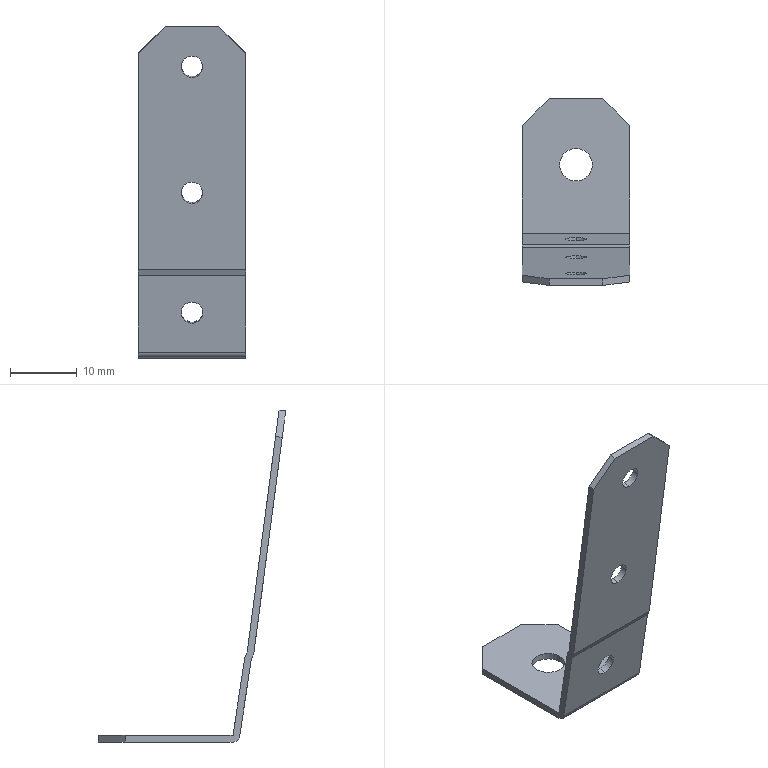Part | SolidWorks | features BaseBody 1 | 1 solid | 25 faces | box 16 x 28.013 x 49.636 mm | volume 1045 mm3 | plane 16 | cylinder 9 | commonest cylinder face diameters 3.2 x6 4.9 x2 2 x1
STEP:
#1=CARTESIAN_POINT('',(-142.,-118.576,-942.719));
#2=VERTEX_POINT('',#1);
#3=CARTESIAN_POINT('',(-142.,-118.159,-945.892));
#4=VERTEX_POINT('',#3);
#5=CARTESIAN_POINT('',(-142.,-118.576,-942.719));
#6=CARTESIAN_POINT('',(-145.2,-118.576,-942.719));
#7=CARTESIAN_POINT('',(-145.2,-118.159,-945.892));
#8=CARTESIAN_POINT('',(-142.,-118.159,-945.892));
#9=(BOUNDED_CURVE()B_SPLINE_CURVE(3,(#5,#6,#7,#8),.UNSPECIFIED.,.F.,.F.)B_SPLINE_CURVE_WITH_KNOTS((4,4),(0.,3.142),.UNSPECIFIED.)CURVE()GEOMETRIC_REPRESENTATION_ITEM()RATIONAL_B_SPLINE_CURVE((1.,0.3333,0.3333,1.))REPRESENTATION_ITEM(''));
#10=EDGE_CURVE('',#2,#4,#9,.T.);
#11=ORIENTED_EDGE('',*,*,#10,.T.);
#12=CARTESIAN_POINT('',(-142.,-117.17,-945.743));
#13=VERTEX_POINT('',#12);
#14=CARTESIAN_POINT('',(-142.,-118.165,-945.893));
#15=DIRECTION('',(0.,0.9888,0.1494));
#16=VECTOR('',#15,1000.);
#17=LINE('',#14,#16);
#18=EDGE_CURVE('',#4,#13,#17,.T.);
#19=ORIENTED_EDGE('',*,*,#18,.T.);
#20=CARTESIAN_POINT('',(-142.,-117.587,-942.57));
#21=VERTEX_POINT('',#20);
#22=CARTESIAN_POINT('',(-142.,-117.17,-945.743));
#23=CARTESIAN_POINT('',(-145.2,-117.17,-945.743));
#24=CARTESIAN_POINT('',(-145.2,-117.587,-942.57));
#25=CARTESIAN_POINT('',(-142.,-117.587,-942.57));
#26=(BOUNDED_CURVE()B_SPLINE_CURVE(3,(#22,#23,#24,#25),.UNSPECIFIED.,.F.,.F.)B_SPLINE_CURVE_WITH_KNOTS((4,4),(3.142,6.283),.UNSPECIFIED.)CURVE()GEOMETRIC_REPRESENTATION_ITEM()RATIONAL_B_SPLINE_CURVE((1.,0.3333,0.3333,1.))REPRESENTATION_ITEM(''));
#27=EDGE_CURVE('',#13,#21,#26,.T.);
#28=ORIENTED_EDGE('',*,*,#27,.T.);
#29=CARTESIAN_POINT('',(-142.,-118.643,-942.729));
#30=DIRECTION('',(0.,0.9888,0.1494));
#31=VECTOR('',#30,1000.);
#32=LINE('',#29,#31);
#33=EDGE_CURVE('',#2,#21,#32,.T.);
#34=ORIENTED_EDGE('',*,*,#33,.F.);
#35=EDGE_LOOP('',(#11,#19,#28,#34));
#36=FACE_OUTER_BOUND('',#35,.T.);
#37=CARTESIAN_POINT('',(-142.,-118.404,-944.311));
#38=DIRECTION('',(0.,0.9888,0.1494));
#39=DIRECTION('',(0.,-0.1494,0.9888));
#40=AXIS2_PLACEMENT_3D('',#37,#38,#39);
#41=CYLINDRICAL_SURFACE('',#40,1.6);
#42=ADVANCED_FACE('',(#36),#41,.F.);
#43=CARTESIAN_POINT('',(-142.,-121.052,-923.878));
#44=VERTEX_POINT('',#43);
#45=CARTESIAN_POINT('',(-142.,-120.635,-927.051));
#46=VERTEX_POINT('',#45);
#47=CARTESIAN_POINT('',(-142.,-121.052,-923.878));
#48=CARTESIAN_POINT('',(-145.2,-121.052,-923.878));
#49=CARTESIAN_POINT('',(-145.2,-120.635,-927.051));
#50=CARTESIAN_POINT('',(-142.,-120.635,-927.051));
#51=(BOUNDED_CURVE()B_SPLINE_CURVE(3,(#47,#48,#49,#50),.UNSPECIFIED.,.F.,.T.)B_SPLINE_CURVE_WITH_KNOTS((4,4),(0.,3.142),.UNSPECIFIED.)CURVE()GEOMETRIC_REPRESENTATION_ITEM()RATIONAL_B_SPLINE_CURVE((1.,0.3333,0.3333,1.))REPRESENTATION_ITEM(''));
#52=EDGE_CURVE('',#44,#46,#51,.T.);
#53=ORIENTED_EDGE('',*,*,#52,.T.);
#54=CARTESIAN_POINT('',(-142.,-119.646,-926.902));
#55=VERTEX_POINT('',#54);
#56=CARTESIAN_POINT('',(-142.,-120.641,-927.052));
#57=DIRECTION('',(0.,0.9888,0.1494));
#58=VECTOR('',#57,1000.);
#59=LINE('',#56,#58);
#60=EDGE_CURVE('',#46,#55,#59,.T.);
#61=ORIENTED_EDGE('',*,*,#60,.T.);
#62=CARTESIAN_POINT('',(-142.,-120.063,-923.728));
#63=VERTEX_POINT('',#62);
#64=CARTESIAN_POINT('',(-142.,-119.646,-926.902));
#65=CARTESIAN_POINT('',(-145.2,-119.646,-926.902));
#66=CARTESIAN_POINT('',(-145.2,-120.063,-923.728));
#67=CARTESIAN_POINT('',(-142.,-120.063,-923.728));
#68=(BOUNDED_CURVE()B_SPLINE_CURVE(3,(#64,#65,#66,#67),.UNSPECIFIED.,.F.,.F.)B_SPLINE_CURVE_WITH_KNOTS((4,4),(3.142,6.283),.UNSPECIFIED.)CURVE()GEOMETRIC_REPRESENTATION_ITEM()RATIONAL_B_SPLINE_CURVE((1.,0.3333,0.3333,1.))REPRESENTATION_ITEM(''));
#69=EDGE_CURVE('',#55,#63,#68,.T.);
#70=ORIENTED_EDGE('',*,*,#69,.T.);
#71=CARTESIAN_POINT('',(-142.,-121.119,-923.888));
#72=DIRECTION('',(0.,0.9888,0.1494));
#73=VECTOR('',#72,1000.);
#74=LINE('',#71,#73);
#75=EDGE_CURVE('',#44,#63,#74,.T.);
#76=ORIENTED_EDGE('',*,*,#75,.F.);
#77=EDGE_LOOP('',(#53,#61,#70,#76));
#78=FACE_OUTER_BOUND('',#77,.T.);
#79=CARTESIAN_POINT('',(-142.,-120.88,-925.47));
#80=DIRECTION('',(0.,0.9888,0.1494));
#81=DIRECTION('',(0.,-0.1494,0.9888));
#82=AXIS2_PLACEMENT_3D('',#79,#80,#81);
#83=CYLINDRICAL_SURFACE('',#82,1.6);
#84=ADVANCED_FACE('',(#78),#83,.F.);
#85=CARTESIAN_POINT('',(-142.,-115.879,-960.636));
#86=VERTEX_POINT('',#85);
#87=CARTESIAN_POINT('',(-142.,-115.401,-963.8));
#88=VERTEX_POINT('',#87);
#89=CARTESIAN_POINT('',(-142.,-115.64,-962.218));
#90=DIRECTION('',(0.,-0.9888,-0.1494));
#91=DIRECTION('',(0.,-0.1494,0.9888));
#92=AXIS2_PLACEMENT_3D('',#89,#90,#91);
#93=CIRCLE('',#92,1.6);
#94=EDGE_CURVE('',#86,#88,#93,.T.);
#95=ORIENTED_EDGE('',*,*,#94,.T.);
#96=CARTESIAN_POINT('',(-142.,-114.412,-963.65));
#97=VERTEX_POINT('',#96);
#98=CARTESIAN_POINT('',(-142.,-115.401,-963.8));
#99=DIRECTION('',(0.,0.9888,0.1494));
#100=VECTOR('',#99,1000.);
#101=LINE('',#98,#100);
#102=EDGE_CURVE('',#88,#97,#101,.T.);
#103=ORIENTED_EDGE('',*,*,#102,.T.);
#104=CARTESIAN_POINT('',(-142.,-114.89,-960.486));
#105=VERTEX_POINT('',#104);
#106=CARTESIAN_POINT('',(-142.,-114.651,-962.068));
#107=DIRECTION('',(0.,0.9888,0.1494));
#108=DIRECTION('',(0.,-0.1494,0.9888));
#109=AXIS2_PLACEMENT_3D('',#106,#107,#108);
#110=CIRCLE('',#109,1.6);
#111=EDGE_CURVE('',#97,#105,#110,.T.);
#112=ORIENTED_EDGE('',*,*,#111,.T.);
#113=CARTESIAN_POINT('',(-142.,-115.879,-960.636));
#114=DIRECTION('',(0.,0.9888,0.1494));
#115=VECTOR('',#114,1000.);
#116=LINE('',#113,#115);
#117=EDGE_CURVE('',#86,#105,#116,.T.);
#118=ORIENTED_EDGE('',*,*,#117,.F.);
#119=EDGE_LOOP('',(#95,#103,#112,#118));
#120=FACE_OUTER_BOUND('',#119,.T.);
#121=CARTESIAN_POINT('',(-142.,-115.64,-962.218));
#122=DIRECTION('',(0.,0.9888,0.1494));
#123=DIRECTION('',(0.,-0.1494,0.9888));
#124=AXIS2_PLACEMENT_3D('',#121,#122,#123);
#125=CYLINDRICAL_SURFACE('',#124,1.6);
#126=ADVANCED_FACE('',(#120),#125,.F.);
#127=CARTESIAN_POINT('',(-139.55,-103.5,-969.001));
#128=VERTEX_POINT('',#127);
#129=CARTESIAN_POINT('',(-144.45,-103.5,-969.001));
#130=VERTEX_POINT('',#129);
#131=CARTESIAN_POINT('',(-142.,-103.5,-969.001));
#132=DIRECTION('',(0.,0.,-1.));
#133=DIRECTION('',(1.,0.,0.));
#134=AXIS2_PLACEMENT_3D('',#131,#132,#133);
#135=CIRCLE('',#134,2.45);
#136=EDGE_CURVE('',#128,#130,#135,.T.);
#137=ORIENTED_EDGE('',*,*,#136,.T.);
#138=CARTESIAN_POINT('',(-144.45,-103.5,-968.001));
#139=VERTEX_POINT('',#138);
#140=CARTESIAN_POINT('',(-144.45,-103.5,-969.001));
#141=DIRECTION('',(0.,0.,1.));
#142=VECTOR('',#141,1000.);
#143=LINE('',#140,#142);
#144=EDGE_CURVE('',#130,#139,#143,.T.);
#145=ORIENTED_EDGE('',*,*,#144,.T.);
#146=CARTESIAN_POINT('',(-139.55,-103.5,-968.001));
#147=VERTEX_POINT('',#146);
#148=CARTESIAN_POINT('',(-142.,-103.5,-968.001));
#149=DIRECTION('',(0.,0.,1.));
#150=DIRECTION('',(1.,0.,0.));
#151=AXIS2_PLACEMENT_3D('',#148,#149,#150);
#152=CIRCLE('',#151,2.45);
#153=EDGE_CURVE('',#139,#147,#152,.T.);
#154=ORIENTED_EDGE('',*,*,#153,.T.);
#155=CARTESIAN_POINT('',(-139.55,-103.5,-969.001));
#156=DIRECTION('',(0.,0.,1.));
#157=VECTOR('',#156,1000.);
#158=LINE('',#155,#157);
#159=EDGE_CURVE('',#128,#147,#158,.T.);
#160=ORIENTED_EDGE('',*,*,#159,.F.);
#161=EDGE_LOOP('',(#137,#145,#154,#160));
#162=FACE_OUTER_BOUND('',#161,.T.);
#163=CARTESIAN_POINT('',(-142.,-103.5,-969.001));
#164=DIRECTION('',(0.,0.,1.));
#165=DIRECTION('',(1.,0.,0.));
#166=AXIS2_PLACEMENT_3D('',#163,#164,#165);
#167=CYLINDRICAL_SURFACE('',#166,2.45);
#168=ADVANCED_FACE('',(#162),#167,.F.);
#169=ORIENTED_EDGE('',*,*,#18,.F.);
#170=CARTESIAN_POINT('',(-142.,-118.159,-945.892));
#171=CARTESIAN_POINT('',(-138.8,-118.159,-945.892));
#172=CARTESIAN_POINT('',(-138.8,-118.576,-942.719));
#173=CARTESIAN_POINT('',(-142.,-118.576,-942.719));
#174=(BOUNDED_CURVE()B_SPLINE_CURVE(3,(#170,#171,#172,#173),.UNSPECIFIED.,.F.,.F.)B_SPLINE_CURVE_WITH_KNOTS((4,4),(3.142,6.283),.UNSPECIFIED.)CURVE()GEOMETRIC_REPRESENTATION_ITEM()RATIONAL_B_SPLINE_CURVE((1.,0.3333,0.3333,1.))REPRESENTATION_ITEM(''));
#175=EDGE_CURVE('',#4,#2,#174,.T.);
#176=ORIENTED_EDGE('',*,*,#175,.T.);
#177=ORIENTED_EDGE('',*,*,#33,.T.);
#178=CARTESIAN_POINT('',(-142.,-117.587,-942.57));
#179=CARTESIAN_POINT('',(-138.8,-117.587,-942.57));
#180=CARTESIAN_POINT('',(-138.8,-117.17,-945.743));
#181=CARTESIAN_POINT('',(-142.,-117.17,-945.743));
#182=(BOUNDED_CURVE()B_SPLINE_CURVE(3,(#178,#179,#180,#181),.UNSPECIFIED.,.F.,.F.)B_SPLINE_CURVE_WITH_KNOTS((4,4),(0.,3.142),.UNSPECIFIED.)CURVE()GEOMETRIC_REPRESENTATION_ITEM()RATIONAL_B_SPLINE_CURVE((1.,0.3333,0.3333,1.))REPRESENTATION_ITEM(''));
#183=EDGE_CURVE('',#21,#13,#182,.T.);
#184=ORIENTED_EDGE('',*,*,#183,.T.);
#185=EDGE_LOOP('',(#169,#176,#177,#184));
#186=FACE_OUTER_BOUND('',#185,.T.);
#187=CARTESIAN_POINT('',(-142.,-118.404,-944.311));
#188=DIRECTION('',(0.,0.9888,0.1494));
#189=DIRECTION('',(0.,-0.1494,0.9888));
#190=AXIS2_PLACEMENT_3D('',#187,#188,#189);
#191=CYLINDRICAL_SURFACE('',#190,1.6);
#192=ADVANCED_FACE('',(#186),#191,.F.);
#193=CARTESIAN_POINT('',(-142.,-120.063,-923.728));
#194=CARTESIAN_POINT('',(-138.8,-120.063,-923.728));
#195=CARTESIAN_POINT('',(-138.8,-119.646,-926.902));
#196=CARTESIAN_POINT('',(-142.,-119.646,-926.902));
#197=(BOUNDED_CURVE()B_SPLINE_CURVE(3,(#193,#194,#195,#196),.UNSPECIFIED.,.F.,.T.)B_SPLINE_CURVE_WITH_KNOTS((4,4),(0.,3.142),.UNSPECIFIED.)CURVE()GEOMETRIC_REPRESENTATION_ITEM()RATIONAL_B_SPLINE_CURVE((1.,0.3333,0.3333,1.))REPRESENTATION_ITEM(''));
#198=EDGE_CURVE('',#63,#55,#197,.T.);
#199=ORIENTED_EDGE('',*,*,#198,.F.);
#200=ORIENTED_EDGE('',*,*,#69,.F.);
#201=EDGE_LOOP('',(#199,#200));
#202=FACE_BOUND('',#201,.T.);
#203=ORIENTED_EDGE('',*,*,#183,.F.);
#204=ORIENTED_EDGE('',*,*,#27,.F.);
#205=EDGE_LOOP('',(#203,#204));
#206=FACE_BOUND('',#205,.T.);
#207=CARTESIAN_POINT('',(-134.,-120.116,-923.331));
#208=VERTEX_POINT('',#207);
#209=CARTESIAN_POINT('',(-138.,-120.637,-919.365));
#210=VERTEX_POINT('',#209);
#211=CARTESIAN_POINT('',(-138.,-120.637,-919.365));
#212=DIRECTION('',(-0.7071,-0.09215,0.7011));
#213=VECTOR('',#212,1000.);
#214=LINE('',#211,#213);
#215=EDGE_CURVE('',#208,#210,#214,.T.);
#216=ORIENTED_EDGE('',*,*,#215,.F.);
#217=CARTESIAN_POINT('',(-134.,-115.881,-955.544));
#218=VERTEX_POINT('',#217);
#219=CARTESIAN_POINT('',(-134.,-118.259,-937.455));
#220=DIRECTION('',(0.,-0.1303,0.9915));
#221=VECTOR('',#220,1000.);
#222=LINE('',#219,#221);
#223=EDGE_CURVE('',#218,#208,#222,.T.);
#224=ORIENTED_EDGE('',*,*,#223,.F.);
#225=CARTESIAN_POINT('',(-150.,-115.881,-955.544));
#226=VERTEX_POINT('',#225);
#227=CARTESIAN_POINT('',(-142.,-115.881,-955.544));
#228=DIRECTION('',(1.,0.,0.));
#229=VECTOR('',#228,1000.);
#230=LINE('',#227,#229);
#231=EDGE_CURVE('',#226,#218,#230,.T.);
#232=ORIENTED_EDGE('',*,*,#231,.F.);
#233=CARTESIAN_POINT('',(-150.,-120.116,-923.331));
#234=VERTEX_POINT('',#233);
#235=CARTESIAN_POINT('',(-150.,-118.259,-937.455));
#236=DIRECTION('',(0.,0.1303,-0.9915));
#237=VECTOR('',#236,1000.);
#238=LINE('',#235,#237);
#239=EDGE_CURVE('',#234,#226,#238,.T.);
#240=ORIENTED_EDGE('',*,*,#239,.F.);
#241=CARTESIAN_POINT('',(-146.,-120.637,-919.365));
#242=VERTEX_POINT('',#241);
#243=CARTESIAN_POINT('',(-150.,-120.116,-923.331));
#244=DIRECTION('',(-0.7071,0.09215,-0.7011));
#245=VECTOR('',#244,1000.);
#246=LINE('',#243,#245);
#247=EDGE_CURVE('',#242,#234,#246,.T.);
#248=ORIENTED_EDGE('',*,*,#247,.F.);
#249=CARTESIAN_POINT('',(-142.,-120.637,-919.365));
#250=DIRECTION('',(-1.,0.,0.));
#251=VECTOR('',#250,1000.);
#252=LINE('',#249,#251);
#253=EDGE_CURVE('',#210,#242,#252,.T.);
#254=ORIENTED_EDGE('',*,*,#253,.F.);
#255=EDGE_LOOP('',(#216,#224,#232,#240,#248,#254));
#256=FACE_OUTER_BOUND('',#255,.T.);
#257=CARTESIAN_POINT('',(-150.,-120.637,-919.365));
#258=DIRECTION('',(0.,-0.9915,-0.1303));
#259=DIRECTION('',(0.,0.1303,-0.9915));
#260=AXIS2_PLACEMENT_3D('',#257,#258,#259);
#261=PLANE('',#260);
#262=ADVANCED_FACE('',(#202,#206,#256),#261,.F.);
#263=ORIENTED_EDGE('',*,*,#52,.F.);
#264=CARTESIAN_POINT('',(-142.,-120.635,-927.051));
#265=CARTESIAN_POINT('',(-138.8,-120.635,-927.051));
#266=CARTESIAN_POINT('',(-138.8,-121.052,-923.878));
#267=CARTESIAN_POINT('',(-142.,-121.052,-923.878));
#268=(BOUNDED_CURVE()B_SPLINE_CURVE(3,(#264,#265,#266,#267),.UNSPECIFIED.,.F.,.F.)B_SPLINE_CURVE_WITH_KNOTS((4,4),(3.142,6.283),.UNSPECIFIED.)CURVE()GEOMETRIC_REPRESENTATION_ITEM()RATIONAL_B_SPLINE_CURVE((1.,0.3333,0.3333,1.))REPRESENTATION_ITEM(''));
#269=EDGE_CURVE('',#46,#44,#268,.T.);
#270=ORIENTED_EDGE('',*,*,#269,.F.);
#271=EDGE_LOOP('',(#263,#270));
#272=FACE_BOUND('',#271,.T.);
#273=ORIENTED_EDGE('',*,*,#10,.F.);
#274=ORIENTED_EDGE('',*,*,#175,.F.);
#275=EDGE_LOOP('',(#273,#274));
#276=FACE_BOUND('',#275,.T.);
#277=CARTESIAN_POINT('',(-138.,-121.628,-919.495));
#278=VERTEX_POINT('',#277);
#279=CARTESIAN_POINT('',(-134.,-121.107,-923.461));
#280=VERTEX_POINT('',#279);
#281=CARTESIAN_POINT('',(-138.,-121.628,-919.495));
#282=DIRECTION('',(0.7071,0.09215,-0.7011));
#283=VECTOR('',#282,1000.);
#284=LINE('',#281,#283);
#285=EDGE_CURVE('',#278,#280,#284,.T.);
#286=ORIENTED_EDGE('',*,*,#285,.F.);
#287=CARTESIAN_POINT('',(-146.,-121.628,-919.495));
#288=VERTEX_POINT('',#287);
#289=CARTESIAN_POINT('',(-142.,-121.628,-919.495));
#290=DIRECTION('',(1.,0.,0.));
#291=VECTOR('',#290,1000.);
#292=LINE('',#289,#291);
#293=EDGE_CURVE('',#288,#278,#292,.T.);
#294=ORIENTED_EDGE('',*,*,#293,.F.);
#295=CARTESIAN_POINT('',(-150.,-121.107,-923.461));
#296=VERTEX_POINT('',#295);
#297=CARTESIAN_POINT('',(-150.,-121.107,-923.461));
#298=DIRECTION('',(0.7071,-0.09215,0.7011));
#299=VECTOR('',#298,1000.);
#300=LINE('',#297,#299);
#301=EDGE_CURVE('',#296,#288,#300,.T.);
#302=ORIENTED_EDGE('',*,*,#301,.F.);
#303=CARTESIAN_POINT('',(-150.,-116.854,-955.821));
#304=VERTEX_POINT('',#303);
#305=CARTESIAN_POINT('',(-150.,-119.241,-937.658));
#306=DIRECTION('',(0.,-0.1303,0.9915));
#307=VECTOR('',#306,1000.);
#308=LINE('',#305,#307);
#309=EDGE_CURVE('',#304,#296,#308,.T.);
#310=ORIENTED_EDGE('',*,*,#309,.F.);
#311=CARTESIAN_POINT('',(-134.,-116.854,-955.821));
#312=VERTEX_POINT('',#311);
#313=CARTESIAN_POINT('',(-142.,-116.854,-955.821));
#314=DIRECTION('',(-1.,0.,0.));
#315=VECTOR('',#314,1000.);
#316=LINE('',#313,#315);
#317=EDGE_CURVE('',#312,#304,#316,.T.);
#318=ORIENTED_EDGE('',*,*,#317,.F.);
#319=CARTESIAN_POINT('',(-134.,-119.241,-937.658));
#320=DIRECTION('',(0.,0.1303,-0.9915));
#321=VECTOR('',#320,1000.);
#322=LINE('',#319,#321);
#323=EDGE_CURVE('',#280,#312,#322,.T.);
#324=ORIENTED_EDGE('',*,*,#323,.F.);
#325=EDGE_LOOP('',(#286,#294,#302,#310,#318,#324));
#326=FACE_OUTER_BOUND('',#325,.T.);
#327=CARTESIAN_POINT('',(-150.,-116.854,-955.821));
#328=DIRECTION('',(0.,0.9915,0.1303));
#329=DIRECTION('',(0.,-0.1303,0.9915));
#330=AXIS2_PLACEMENT_3D('',#327,#328,#329);
#331=PLANE('',#330);
#332=ADVANCED_FACE('',(#272,#276,#326),#331,.F.);
#333=ORIENTED_EDGE('',*,*,#60,.F.);
#334=ORIENTED_EDGE('',*,*,#269,.T.);
#335=ORIENTED_EDGE('',*,*,#75,.T.);
#336=ORIENTED_EDGE('',*,*,#198,.T.);
#337=EDGE_LOOP('',(#333,#334,#335,#336));
#338=FACE_OUTER_BOUND('',#337,.T.);
#339=CARTESIAN_POINT('',(-142.,-120.88,-925.47));
#340=DIRECTION('',(0.,0.9888,0.1494));
#341=DIRECTION('',(0.,-0.1494,0.9888));
#342=AXIS2_PLACEMENT_3D('',#339,#340,#341);
#343=CYLINDRICAL_SURFACE('',#342,1.6);
#344=ADVANCED_FACE('',(#338),#343,.F.);
#345=CARTESIAN_POINT('',(-138.,-121.133,-919.43));
#346=DIRECTION('',(0.,-0.9915,-0.1303));
#347=VECTOR('',#346,1000.);
#348=LINE('',#345,#347);
#349=EDGE_CURVE('',#210,#278,#348,.T.);
#350=ORIENTED_EDGE('',*,*,#349,.F.);
#351=ORIENTED_EDGE('',*,*,#253,.T.);
#352=CARTESIAN_POINT('',(-146.,-121.133,-919.43));
#353=DIRECTION('',(0.,0.9915,0.1303));
#354=VECTOR('',#353,1000.);
#355=LINE('',#352,#354);
#356=EDGE_CURVE('',#288,#242,#355,.T.);
#357=ORIENTED_EDGE('',*,*,#356,.F.);
#358=ORIENTED_EDGE('',*,*,#293,.T.);
#359=EDGE_LOOP('',(#350,#351,#357,#358));
#360=FACE_OUTER_BOUND('',#359,.T.);
#361=CARTESIAN_POINT('',(-146.,-121.628,-919.495));
#362=DIRECTION('',(0.,0.1303,-0.9915));
#363=DIRECTION('',(0.,0.9915,0.1303));
#364=AXIS2_PLACEMENT_3D('',#361,#362,#363);
#365=PLANE('',#364);
#366=ADVANCED_FACE('',(#360),#365,.F.);
#367=ORIENTED_EDGE('',*,*,#215,.T.);
#368=ORIENTED_EDGE('',*,*,#349,.T.);
#369=ORIENTED_EDGE('',*,*,#285,.T.);
#370=CARTESIAN_POINT('',(-134.,-120.611,-923.396));
#371=DIRECTION('',(0.,0.9915,0.1303));
#372=VECTOR('',#371,1000.);
#373=LINE('',#370,#372);
#374=EDGE_CURVE('',#280,#208,#373,.T.);
#375=ORIENTED_EDGE('',*,*,#374,.T.);
#376=EDGE_LOOP('',(#367,#368,#369,#375));
#377=FACE_OUTER_BOUND('',#376,.T.);
#378=CARTESIAN_POINT('',(-138.,-120.637,-919.365));
#379=DIRECTION('',(0.7071,-0.09215,0.7011));
#380=DIRECTION('',(0.,-0.9915,-0.1303));
#381=AXIS2_PLACEMENT_3D('',#378,#379,#380);
#382=PLANE('',#381);
#383=ADVANCED_FACE('',(#377),#382,.T.);
#384=CARTESIAN_POINT('',(-134.,-113.755,-968.001));
#385=VERTEX_POINT('',#384);
#386=CARTESIAN_POINT('',(-134.,-115.513,-956.362));
#387=VERTEX_POINT('',#386);
#388=CARTESIAN_POINT('',(-134.,-113.755,-968.001));
#389=DIRECTION('',(0.,-0.1494,0.9888));
#390=VECTOR('',#389,1000.);
#391=LINE('',#388,#390);
#392=EDGE_CURVE('',#385,#387,#391,.T.);
#393=ORIENTED_EDGE('',*,*,#392,.T.);
#394=CARTESIAN_POINT('',(-134.,-115.513,-956.362));
#395=DIRECTION('',(0.,-0.4107,0.9118));
#396=VECTOR('',#395,1000.);
#397=LINE('',#394,#396);
#398=EDGE_CURVE('',#387,#218,#397,.T.);
#399=ORIENTED_EDGE('',*,*,#398,.T.);
#400=ORIENTED_EDGE('',*,*,#223,.T.);
#401=ORIENTED_EDGE('',*,*,#374,.F.);
#402=ORIENTED_EDGE('',*,*,#323,.T.);
#403=CARTESIAN_POINT('',(-134.,-116.481,-956.647));
#404=VERTEX_POINT('',#403);
#405=CARTESIAN_POINT('',(-134.,-116.854,-955.821));
#406=DIRECTION('',(0.,0.4107,-0.9118));
#407=VECTOR('',#406,1000.);
#408=LINE('',#405,#407);
#409=EDGE_CURVE('',#312,#404,#408,.T.);
#410=ORIENTED_EDGE('',*,*,#409,.T.);
#411=CARTESIAN_POINT('',(-134.,-114.744,-968.15));
#412=VERTEX_POINT('',#411);
#413=CARTESIAN_POINT('',(-134.,-116.481,-956.647));
#414=DIRECTION('',(0.,0.1494,-0.9888));
#415=VECTOR('',#414,1000.);
#416=LINE('',#413,#415);
#417=EDGE_CURVE('',#404,#412,#416,.T.);
#418=ORIENTED_EDGE('',*,*,#417,.T.);
#419=CARTESIAN_POINT('',(-134.,-113.755,-969.001));
#420=VERTEX_POINT('',#419);
#421=CARTESIAN_POINT('',(-134.,-113.755,-968.001));
#422=DIRECTION('',(1.,0.,0.));
#423=DIRECTION('',(0.,0.,-1.));
#424=AXIS2_PLACEMENT_3D('',#421,#422,#423);
#425=CIRCLE('',#424,1.);
#426=EDGE_CURVE('',#412,#420,#425,.T.);
#427=ORIENTED_EDGE('',*,*,#426,.T.);
#428=CARTESIAN_POINT('',(-134.,-97.615,-969.001));
#429=VERTEX_POINT('',#428);
#430=CARTESIAN_POINT('',(-134.,-109.432,-969.001));
#431=DIRECTION('',(0.,1.,0.));
#432=VECTOR('',#431,1000.);
#433=LINE('',#430,#432);
#434=EDGE_CURVE('',#420,#429,#433,.T.);
#435=ORIENTED_EDGE('',*,*,#434,.T.);
#436=CARTESIAN_POINT('',(-134.,-97.615,-968.001));
#437=VERTEX_POINT('',#436);
#438=CARTESIAN_POINT('',(-134.,-97.615,-968.501));
#439=DIRECTION('',(0.,0.,-1.));
#440=VECTOR('',#439,1000.);
#441=LINE('',#438,#440);
#442=EDGE_CURVE('',#437,#429,#441,.T.);
#443=ORIENTED_EDGE('',*,*,#442,.F.);
#444=CARTESIAN_POINT('',(-134.,-109.432,-968.001));
#445=DIRECTION('',(0.,-1.,0.));
#446=VECTOR('',#445,1000.);
#447=LINE('',#444,#446);
#448=EDGE_CURVE('',#437,#385,#447,.T.);
#449=ORIENTED_EDGE('',*,*,#448,.T.);
#450=EDGE_LOOP('',(#393,#399,#400,#401,#402,#410,#418,#427,#435,#443,#449));
#451=FACE_OUTER_BOUND('',#450,.T.);
#452=CARTESIAN_POINT('',(-134.,-121.248,-923.057));
#453=DIRECTION('',(1.,0.,0.));
#454=DIRECTION('',(0.,0.,-1.));
#455=AXIS2_PLACEMENT_3D('',#452,#453,#454);
#456=PLANE('',#455);
#457=ADVANCED_FACE('',(#451),#456,.T.);
#458=CARTESIAN_POINT('',(-150.,-115.513,-956.362));
#459=VERTEX_POINT('',#458);
#460=CARTESIAN_POINT('',(-142.,-115.513,-956.362));
#461=DIRECTION('',(1.,0.,0.));
#462=VECTOR('',#461,1000.);
#463=LINE('',#460,#462);
#464=EDGE_CURVE('',#459,#387,#463,.T.);
#465=ORIENTED_EDGE('',*,*,#464,.F.);
#466=CARTESIAN_POINT('',(-150.,-115.697,-955.953));
#467=DIRECTION('',(0.,0.4107,-0.9118));
#468=VECTOR('',#467,1000.);
#469=LINE('',#466,#468);
#470=EDGE_CURVE('',#226,#459,#469,.T.);
#471=ORIENTED_EDGE('',*,*,#470,.F.);
#472=ORIENTED_EDGE('',*,*,#231,.T.);
#473=ORIENTED_EDGE('',*,*,#398,.F.);
#474=EDGE_LOOP('',(#465,#471,#472,#473));
#475=FACE_OUTER_BOUND('',#474,.T.);
#476=CARTESIAN_POINT('',(-150.,-115.881,-955.544));
#477=DIRECTION('',(0.,-0.9118,-0.4107));
#478=DIRECTION('',(0.,0.4107,-0.9118));
#479=AXIS2_PLACEMENT_3D('',#476,#477,#478);
#480=PLANE('',#479);
#481=ADVANCED_FACE('',(#475),#480,.F.);
#482=CARTESIAN_POINT('',(-150.,-121.107,-923.461));
#483=DIRECTION('',(0.,-0.9915,-0.1303));
#484=VECTOR('',#483,1000.);
#485=LINE('',#482,#484);
#486=EDGE_CURVE('',#234,#296,#485,.T.);
#487=ORIENTED_EDGE('',*,*,#486,.F.);
#488=ORIENTED_EDGE('',*,*,#239,.T.);
#489=ORIENTED_EDGE('',*,*,#470,.T.);
#490=CARTESIAN_POINT('',(-150.,-113.755,-968.001));
#491=VERTEX_POINT('',#490);
#492=CARTESIAN_POINT('',(-150.,-115.513,-956.362));
#493=DIRECTION('',(0.,-0.1494,0.9888));
#494=VECTOR('',#493,1000.);
#495=LINE('',#492,#494);
#496=EDGE_CURVE('',#491,#459,#495,.T.);
#497=ORIENTED_EDGE('',*,*,#496,.F.);
#498=CARTESIAN_POINT('',(-150.,-97.615,-968.001));
#499=VERTEX_POINT('',#498);
#500=CARTESIAN_POINT('',(-150.,-109.432,-968.001));
#501=DIRECTION('',(0.,-1.,0.));
#502=VECTOR('',#501,1000.);
#503=LINE('',#500,#502);
#504=EDGE_CURVE('',#499,#491,#503,.T.);
#505=ORIENTED_EDGE('',*,*,#504,.F.);
#506=CARTESIAN_POINT('',(-150.,-97.615,-969.001));
#507=VERTEX_POINT('',#506);
#508=CARTESIAN_POINT('',(-150.,-97.615,-968.501));
#509=DIRECTION('',(0.,0.,-1.));
#510=VECTOR('',#509,1000.);
#511=LINE('',#508,#510);
#512=EDGE_CURVE('',#499,#507,#511,.T.);
#513=ORIENTED_EDGE('',*,*,#512,.T.);
#514=CARTESIAN_POINT('',(-150.,-113.755,-969.001));
#515=VERTEX_POINT('',#514);
#516=CARTESIAN_POINT('',(-150.,-109.432,-969.001));
#517=DIRECTION('',(0.,1.,0.));
#518=VECTOR('',#517,1000.);
#519=LINE('',#516,#518);
#520=EDGE_CURVE('',#515,#507,#519,.T.);
#521=ORIENTED_EDGE('',*,*,#520,.F.);
#522=CARTESIAN_POINT('',(-150.,-114.744,-968.15));
#523=VERTEX_POINT('',#522);
#524=CARTESIAN_POINT('',(-150.,-113.755,-968.001));
#525=DIRECTION('',(-1.,0.,0.));
#526=DIRECTION('',(0.,0.,-1.));
#527=AXIS2_PLACEMENT_3D('',#524,#525,#526);
#528=CIRCLE('',#527,1.);
#529=EDGE_CURVE('',#515,#523,#528,.T.);
#530=ORIENTED_EDGE('',*,*,#529,.T.);
#531=CARTESIAN_POINT('',(-150.,-116.481,-956.647));
#532=VERTEX_POINT('',#531);
#533=CARTESIAN_POINT('',(-150.,-114.744,-968.15));
#534=DIRECTION('',(0.,0.1494,-0.9888));
#535=VECTOR('',#534,1000.);
#536=LINE('',#533,#535);
#537=EDGE_CURVE('',#532,#523,#536,.T.);
#538=ORIENTED_EDGE('',*,*,#537,.F.);
#539=CARTESIAN_POINT('',(-150.,-116.481,-956.647));
#540=DIRECTION('',(0.,0.4107,-0.9118));
#541=VECTOR('',#540,1000.);
#542=LINE('',#539,#541);
#543=EDGE_CURVE('',#304,#532,#542,.T.);
#544=ORIENTED_EDGE('',*,*,#543,.F.);
#545=ORIENTED_EDGE('',*,*,#309,.T.);
#546=EDGE_LOOP('',(#487,#488,#489,#497,#505,#513,#521,#530,#538,#544,#545));
#547=FACE_OUTER_BOUND('',#546,.T.);
#548=CARTESIAN_POINT('',(-150.,-121.248,-923.057));
#549=DIRECTION('',(1.,0.,0.));
#550=DIRECTION('',(0.,0.,-1.));
#551=AXIS2_PLACEMENT_3D('',#548,#549,#550);
#552=PLANE('',#551);
#553=ADVANCED_FACE('',(#547),#552,.F.);
#554=ORIENTED_EDGE('',*,*,#356,.T.);
#555=ORIENTED_EDGE('',*,*,#247,.T.);
#556=ORIENTED_EDGE('',*,*,#486,.T.);
#557=ORIENTED_EDGE('',*,*,#301,.T.);
#558=EDGE_LOOP('',(#554,#555,#556,#557));
#559=FACE_OUTER_BOUND('',#558,.T.);
#560=CARTESIAN_POINT('',(-150.,-121.107,-923.461));
#561=DIRECTION('',(0.7071,0.09215,-0.7011));
#562=DIRECTION('',(0.,0.9915,0.1303));
#563=AXIS2_PLACEMENT_3D('',#560,#561,#562);
#564=PLANE('',#563);
#565=ADVANCED_FACE('',(#559),#564,.F.);
#566=ORIENTED_EDGE('',*,*,#317,.T.);
#567=ORIENTED_EDGE('',*,*,#543,.T.);
#568=CARTESIAN_POINT('',(-142.,-116.481,-956.647));
#569=DIRECTION('',(-1.,0.,0.));
#570=VECTOR('',#569,1000.);
#571=LINE('',#568,#570);
#572=EDGE_CURVE('',#404,#532,#571,.T.);
#573=ORIENTED_EDGE('',*,*,#572,.F.);
#574=ORIENTED_EDGE('',*,*,#409,.F.);
#575=EDGE_LOOP('',(#566,#567,#573,#574));
#576=FACE_OUTER_BOUND('',#575,.T.);
#577=CARTESIAN_POINT('',(-150.,-116.481,-956.647));
#578=DIRECTION('',(0.,0.9118,0.4107));
#579=DIRECTION('',(0.,-0.4107,0.9118));
#580=AXIS2_PLACEMENT_3D('',#577,#578,#579);
#581=PLANE('',#580);
#582=ADVANCED_FACE('',(#576),#581,.F.);
#583=CARTESIAN_POINT('',(-142.,-114.651,-962.068));
#584=DIRECTION('',(0.,0.9888,0.1494));
#585=DIRECTION('',(0.,-0.1494,0.9888));
#586=AXIS2_PLACEMENT_3D('',#583,#584,#585);
#587=CIRCLE('',#586,1.6);
#588=EDGE_CURVE('',#105,#97,#587,.T.);
#589=ORIENTED_EDGE('',*,*,#588,.F.);
#590=ORIENTED_EDGE('',*,*,#111,.F.);
#591=EDGE_LOOP('',(#589,#590));
#592=FACE_BOUND('',#591,.T.);
#593=CARTESIAN_POINT('',(-142.,-113.755,-968.001));
#594=DIRECTION('',(1.,0.,0.));
#595=VECTOR('',#594,1000.);
#596=LINE('',#593,#595);
#597=EDGE_CURVE('',#491,#385,#596,.T.);
#598=ORIENTED_EDGE('',*,*,#597,.F.);
#599=ORIENTED_EDGE('',*,*,#496,.T.);
#600=ORIENTED_EDGE('',*,*,#464,.T.);
#601=ORIENTED_EDGE('',*,*,#392,.F.);
#602=EDGE_LOOP('',(#598,#599,#600,#601));
#603=FACE_OUTER_BOUND('',#602,.T.);
#604=CARTESIAN_POINT('',(-150.,-115.513,-956.362));
#605=DIRECTION('',(0.,-0.9888,-0.1494));
#606=DIRECTION('',(0.,0.1494,-0.9888));
#607=AXIS2_PLACEMENT_3D('',#604,#605,#606);
#608=PLANE('',#607);
#609=ADVANCED_FACE('',(#592,#603),#608,.F.);
#610=CARTESIAN_POINT('',(-142.,-103.5,-968.001));
#611=DIRECTION('',(0.,0.,1.));
#612=DIRECTION('',(1.,0.,0.));
#613=AXIS2_PLACEMENT_3D('',#610,#611,#612);
#614=CIRCLE('',#613,2.45);
#615=EDGE_CURVE('',#147,#139,#614,.T.);
#616=ORIENTED_EDGE('',*,*,#615,.F.);
#617=ORIENTED_EDGE('',*,*,#153,.F.);
#618=EDGE_LOOP('',(#616,#617));
#619=FACE_BOUND('',#618,.T.);
#620=CARTESIAN_POINT('',(-138.,-93.615,-968.001));
#621=VERTEX_POINT('',#620);
#622=CARTESIAN_POINT('',(-138.,-93.615,-968.001));
#623=DIRECTION('',(0.7071,-0.7071,0.));
#624=VECTOR('',#623,1000.);
#625=LINE('',#622,#624);
#626=EDGE_CURVE('',#621,#437,#625,.T.);
#627=ORIENTED_EDGE('',*,*,#626,.F.);
#628=CARTESIAN_POINT('',(-146.,-93.615,-968.001));
#629=VERTEX_POINT('',#628);
#630=CARTESIAN_POINT('',(-142.,-93.615,-968.001));
#631=DIRECTION('',(1.,0.,0.));
#632=VECTOR('',#631,1000.);
#633=LINE('',#630,#632);
#634=EDGE_CURVE('',#629,#621,#633,.T.);
#635=ORIENTED_EDGE('',*,*,#634,.F.);
#636=CARTESIAN_POINT('',(-150.,-97.615,-968.001));
#637=DIRECTION('',(0.7071,0.7071,0.));
#638=VECTOR('',#637,1000.);
#639=LINE('',#636,#638);
#640=EDGE_CURVE('',#499,#629,#639,.T.);
#641=ORIENTED_EDGE('',*,*,#640,.F.);
#642=ORIENTED_EDGE('',*,*,#504,.T.);
#643=ORIENTED_EDGE('',*,*,#597,.T.);
#644=ORIENTED_EDGE('',*,*,#448,.F.);
#645=EDGE_LOOP('',(#627,#635,#641,#642,#643,#644));
#646=FACE_OUTER_BOUND('',#645,.T.);
#647=CARTESIAN_POINT('',(-134.,-113.755,-968.001));
#648=DIRECTION('',(0.,0.,-1.));
#649=DIRECTION('',(-1.,0.,0.));
#650=AXIS2_PLACEMENT_3D('',#647,#648,#649);
#651=PLANE('',#650);
#652=ADVANCED_FACE('',(#619,#646),#651,.F.);
#653=ORIENTED_EDGE('',*,*,#136,.F.);
#654=CARTESIAN_POINT('',(-142.,-103.5,-969.001));
#655=DIRECTION('',(0.,0.,-1.));
#656=DIRECTION('',(1.,0.,0.));
#657=AXIS2_PLACEMENT_3D('',#654,#655,#656);
#658=CIRCLE('',#657,2.45);
#659=EDGE_CURVE('',#130,#128,#658,.T.);
#660=ORIENTED_EDGE('',*,*,#659,.F.);
#661=EDGE_LOOP('',(#653,#660));
#662=FACE_BOUND('',#661,.T.);
#663=CARTESIAN_POINT('',(-138.,-93.615,-969.001));
#664=VERTEX_POINT('',#663);
#665=CARTESIAN_POINT('',(-138.,-93.615,-969.001));
#666=DIRECTION('',(-0.7071,0.7071,0.));
#667=VECTOR('',#666,1000.);
#668=LINE('',#665,#667);
#669=EDGE_CURVE('',#429,#664,#668,.T.);
#670=ORIENTED_EDGE('',*,*,#669,.F.);
#671=ORIENTED_EDGE('',*,*,#434,.F.);
#672=CARTESIAN_POINT('',(-142.,-113.755,-969.001));
#673=DIRECTION('',(1.,0.,0.));
#674=VECTOR('',#673,1000.);
#675=LINE('',#672,#674);
#676=EDGE_CURVE('',#515,#420,#675,.T.);
#677=ORIENTED_EDGE('',*,*,#676,.F.);
#678=ORIENTED_EDGE('',*,*,#520,.T.);
#679=CARTESIAN_POINT('',(-146.,-93.615,-969.001));
#680=VERTEX_POINT('',#679);
#681=CARTESIAN_POINT('',(-150.,-97.615,-969.001));
#682=DIRECTION('',(-0.7071,-0.7071,0.));
#683=VECTOR('',#682,1000.);
#684=LINE('',#681,#683);
#685=EDGE_CURVE('',#680,#507,#684,.T.);
#686=ORIENTED_EDGE('',*,*,#685,.F.);
#687=CARTESIAN_POINT('',(-142.,-93.615,-969.001));
#688=DIRECTION('',(-1.,0.,0.));
#689=VECTOR('',#688,1000.);
#690=LINE('',#687,#689);
#691=EDGE_CURVE('',#664,#680,#690,.T.);
#692=ORIENTED_EDGE('',*,*,#691,.F.);
#693=EDGE_LOOP('',(#670,#671,#677,#678,#686,#692));
#694=FACE_OUTER_BOUND('',#693,.T.);
#695=CARTESIAN_POINT('',(-150.,-113.755,-969.001));
#696=DIRECTION('',(0.,0.,1.));
#697=DIRECTION('',(1.,0.,0.));
#698=AXIS2_PLACEMENT_3D('',#695,#696,#697);
#699=PLANE('',#698);
#700=ADVANCED_FACE('',(#662,#694),#699,.F.);
#701=ORIENTED_EDGE('',*,*,#94,.F.);
#702=CARTESIAN_POINT('',(-142.,-115.64,-962.218));
#703=DIRECTION('',(0.,-0.9888,-0.1494));
#704=DIRECTION('',(0.,-0.1494,0.9888));
#705=AXIS2_PLACEMENT_3D('',#702,#703,#704);
#706=CIRCLE('',#705,1.6);
#707=EDGE_CURVE('',#88,#86,#706,.T.);
#708=ORIENTED_EDGE('',*,*,#707,.F.);
#709=EDGE_LOOP('',(#701,#708));
#710=FACE_BOUND('',#709,.T.);
#711=ORIENTED_EDGE('',*,*,#572,.T.);
#712=ORIENTED_EDGE('',*,*,#537,.T.);
#713=CARTESIAN_POINT('',(-142.,-114.744,-968.15));
#714=DIRECTION('',(-1.,0.,0.));
#715=VECTOR('',#714,1000.);
#716=LINE('',#713,#715);
#717=EDGE_CURVE('',#412,#523,#716,.T.);
#718=ORIENTED_EDGE('',*,*,#717,.F.);
#719=ORIENTED_EDGE('',*,*,#417,.F.);
#720=EDGE_LOOP('',(#711,#712,#718,#719));
#721=FACE_OUTER_BOUND('',#720,.T.);
#722=CARTESIAN_POINT('',(-150.,-114.744,-968.15));
#723=DIRECTION('',(0.,0.9888,0.1494));
#724=DIRECTION('',(0.,-0.1494,0.9888));
#725=AXIS2_PLACEMENT_3D('',#722,#723,#724);
#726=PLANE('',#725);
#727=ADVANCED_FACE('',(#710,#721),#726,.F.);
#728=ORIENTED_EDGE('',*,*,#102,.F.);
#729=ORIENTED_EDGE('',*,*,#707,.T.);
#730=ORIENTED_EDGE('',*,*,#117,.T.);
#731=ORIENTED_EDGE('',*,*,#588,.T.);
#732=EDGE_LOOP('',(#728,#729,#730,#731));
#733=FACE_OUTER_BOUND('',#732,.T.);
#734=CARTESIAN_POINT('',(-142.,-115.64,-962.218));
#735=DIRECTION('',(0.,0.9888,0.1494));
#736=DIRECTION('',(0.,-0.1494,0.9888));
#737=AXIS2_PLACEMENT_3D('',#734,#735,#736);
#738=CYLINDRICAL_SURFACE('',#737,1.6);
#739=ADVANCED_FACE('',(#733),#738,.F.);
#740=ORIENTED_EDGE('',*,*,#144,.F.);
#741=ORIENTED_EDGE('',*,*,#659,.T.);
#742=ORIENTED_EDGE('',*,*,#159,.T.);
#743=ORIENTED_EDGE('',*,*,#615,.T.);
#744=EDGE_LOOP('',(#740,#741,#742,#743));
#745=FACE_OUTER_BOUND('',#744,.T.);
#746=CARTESIAN_POINT('',(-142.,-103.5,-969.001));
#747=DIRECTION('',(0.,0.,1.));
#748=DIRECTION('',(1.,0.,0.));
#749=AXIS2_PLACEMENT_3D('',#746,#747,#748);
#750=CYLINDRICAL_SURFACE('',#749,2.45);
#751=ADVANCED_FACE('',(#745),#750,.F.);
#752=ORIENTED_EDGE('',*,*,#669,.T.);
#753=CARTESIAN_POINT('',(-138.,-93.615,-968.501));
#754=DIRECTION('',(0.,0.,1.));
#755=VECTOR('',#754,1000.);
#756=LINE('',#753,#755);
#757=EDGE_CURVE('',#664,#621,#756,.T.);
#758=ORIENTED_EDGE('',*,*,#757,.T.);
#759=ORIENTED_EDGE('',*,*,#626,.T.);
#760=ORIENTED_EDGE('',*,*,#442,.T.);
#761=EDGE_LOOP('',(#752,#758,#759,#760));
#762=FACE_OUTER_BOUND('',#761,.T.);
#763=CARTESIAN_POINT('',(-138.,-93.615,-969.001));
#764=DIRECTION('',(0.7071,0.7071,0.));
#765=DIRECTION('',(0.,0.,1.));
#766=AXIS2_PLACEMENT_3D('',#763,#764,#765);
#767=PLANE('',#766);
#768=ADVANCED_FACE('',(#762),#767,.T.);
#769=ORIENTED_EDGE('',*,*,#757,.F.);
#770=ORIENTED_EDGE('',*,*,#691,.T.);
#771=CARTESIAN_POINT('',(-146.,-93.615,-968.501));
#772=DIRECTION('',(0.,0.,-1.));
#773=VECTOR('',#772,1000.);
#774=LINE('',#771,#773);
#775=EDGE_CURVE('',#629,#680,#774,.T.);
#776=ORIENTED_EDGE('',*,*,#775,.F.);
#777=ORIENTED_EDGE('',*,*,#634,.T.);
#778=EDGE_LOOP('',(#769,#770,#776,#777));
#779=FACE_OUTER_BOUND('',#778,.T.);
#780=CARTESIAN_POINT('',(-146.,-93.615,-968.001));
#781=DIRECTION('',(0.,-1.,0.));
#782=DIRECTION('',(0.,0.,-1.));
#783=AXIS2_PLACEMENT_3D('',#780,#781,#782);
#784=PLANE('',#783);
#785=ADVANCED_FACE('',(#779),#784,.F.);
#786=ORIENTED_EDGE('',*,*,#775,.T.);
#787=ORIENTED_EDGE('',*,*,#685,.T.);
#788=ORIENTED_EDGE('',*,*,#512,.F.);
#789=ORIENTED_EDGE('',*,*,#640,.T.);
#790=EDGE_LOOP('',(#786,#787,#788,#789));
#791=FACE_OUTER_BOUND('',#790,.T.);
#792=CARTESIAN_POINT('',(-150.,-97.615,-968.001));
#793=DIRECTION('',(0.7071,-0.7071,0.));
#794=DIRECTION('',(0.,0.,-1.));
#795=AXIS2_PLACEMENT_3D('',#792,#793,#794);
#796=PLANE('',#795);
#797=ADVANCED_FACE('',(#791),#796,.F.);
#798=ORIENTED_EDGE('',*,*,#717,.T.);
#799=ORIENTED_EDGE('',*,*,#529,.F.);
#800=ORIENTED_EDGE('',*,*,#676,.T.);
#801=ORIENTED_EDGE('',*,*,#426,.F.);
#802=EDGE_LOOP('',(#798,#799,#800,#801));
#803=FACE_OUTER_BOUND('',#802,.T.);
#804=CARTESIAN_POINT('',(-150.,-113.755,-968.001));
#805=DIRECTION('',(1.,0.,0.));
#806=DIRECTION('',(0.,0.,-1.));
#807=AXIS2_PLACEMENT_3D('',#804,#805,#806);
#808=CYLINDRICAL_SURFACE('',#807,1.);
#809=ADVANCED_FACE('',(#803),#808,.T.);
#810=CLOSED_SHELL('',(#42,#84,#126,#168,#192,#262,#332,#344,#366,#383,#457,#481,#553,#565,#582,#609,#652,#700,#727,#739,#751,#768,#785,#797,#809));
#811=MANIFOLD_SOLID_BREP('',#810);
#812=CARTESIAN_POINT('',(0.,0.,0.));
#813=DIRECTION('',(0.,0.,1.));
#814=DIRECTION('',(1.,0.,0.));
#815=AXIS2_PLACEMENT_3D('',#812,#813,#814);
#816=(LENGTH_UNIT()NAMED_UNIT(*)SI_UNIT(.MILLI.,.METRE.));
#817=UNCERTAINTY_MEASURE_WITH_UNIT(LENGTH_MEASURE(0.00001),#816,'','');
#818=(NAMED_UNIT(*)PLANE_ANGLE_UNIT()SI_UNIT($,.RADIAN.));
#819=(NAMED_UNIT(*)SI_UNIT($,.STERADIAN.)SOLID_ANGLE_UNIT());
#820=(GEOMETRIC_REPRESENTATION_CONTEXT(3)GLOBAL_UNCERTAINTY_ASSIGNED_CONTEXT((#817))GLOBAL_UNIT_ASSIGNED_CONTEXT((#816,#818,#819))REPRESENTATION_CONTEXT('',''));
#821=ADVANCED_BREP_SHAPE_REPRESENTATION('',(#811,#815),#820);